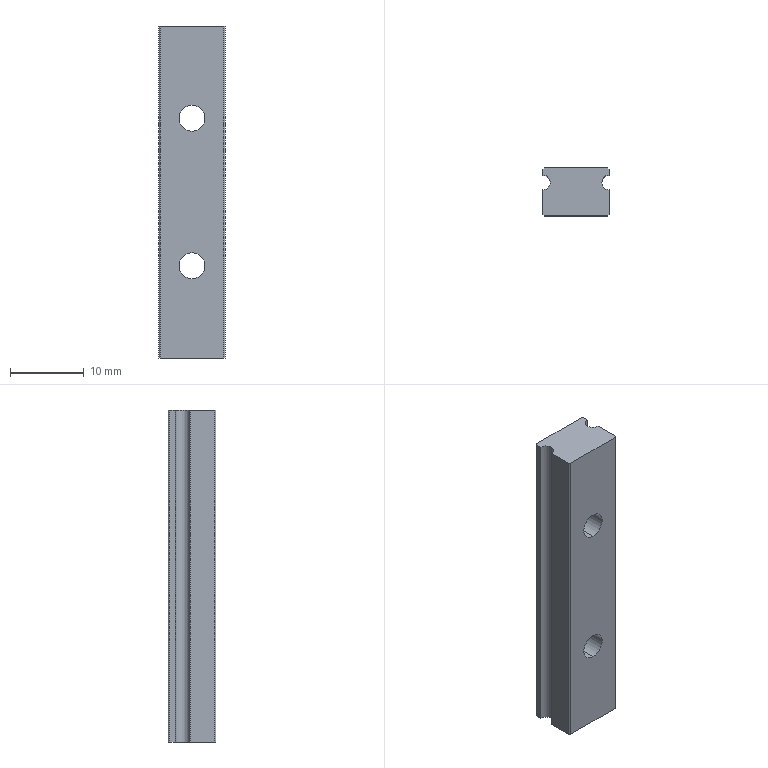Part | STEP file | 1 solid | 25 faces | box 9 x 6.5 x 45 mm | volume 2232 mm3 | plane 14 | cylinder 11 | commonest cylinder face diameters 3.5 x4 6 x4 2 x3